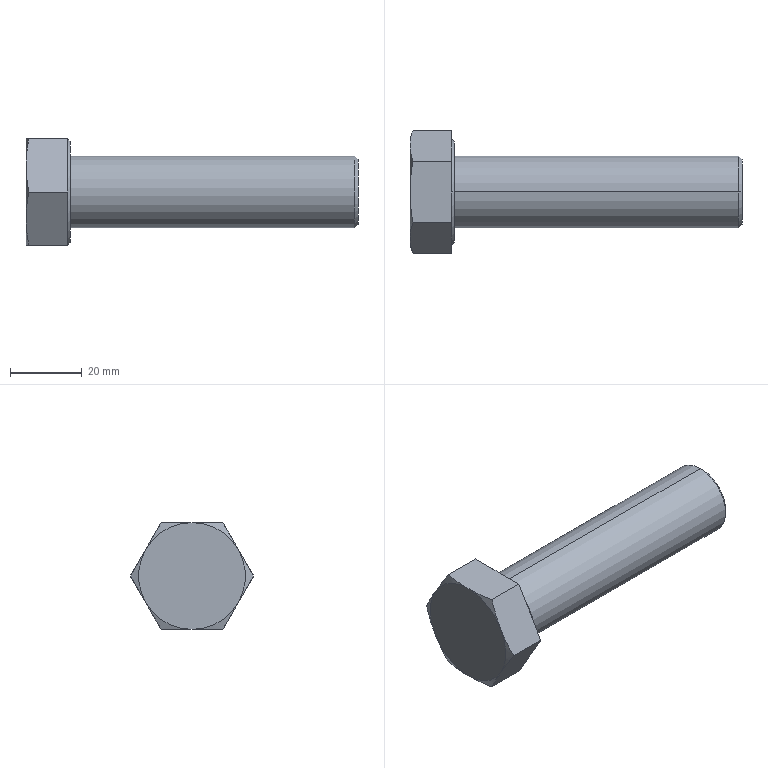Part | SolidWorks | features RevCut 3, Boss 1, Chamfer 1, Extrusion 1, Fillet 1, LPattern 1 | 1 solid | 27 faces | box 92.28 x 34.26 x 29.67 mm | volume 34365 mm3 | plane 15 | cone 10 | cylinder 2 | commonest cylinder face diameters 20 x2
STEP:
#1=CARTESIAN_POINT('',(92.28,0.,-9.));
#2=VERTEX_POINT('',#1);
#3=CARTESIAN_POINT('',(92.28,0.,9.));
#4=VERTEX_POINT('',#3);
#5=CARTESIAN_POINT('',(92.28,0.,0.));
#6=DIRECTION('',(1.,0.,0.));
#7=DIRECTION('',(0.,0.,-1.));
#8=AXIS2_PLACEMENT_3D('',#5,#6,#7);
#9=CIRCLE('',#8,9.);
#10=EDGE_CURVE('',#2,#4,#9,.T.);
#11=ORIENTED_EDGE('',*,*,#10,.F.);
#12=CARTESIAN_POINT('',(91.28,0.,-10.));
#13=VERTEX_POINT('',#12);
#14=CARTESIAN_POINT('',(92.28,0.,-9.));
#15=DIRECTION('',(-0.7071,0.,-0.7071));
#16=VECTOR('',#15,1000.);
#17=LINE('',#14,#16);
#18=EDGE_CURVE('',#2,#13,#17,.T.);
#19=ORIENTED_EDGE('',*,*,#18,.T.);
#20=CARTESIAN_POINT('',(91.28,0.,10.));
#21=VERTEX_POINT('',#20);
#22=CARTESIAN_POINT('',(91.28,0.,0.));
#23=DIRECTION('',(-1.,0.,0.));
#24=DIRECTION('',(0.,0.,-1.));
#25=AXIS2_PLACEMENT_3D('',#22,#23,#24);
#26=CIRCLE('',#25,10.);
#27=EDGE_CURVE('',#21,#13,#26,.T.);
#28=ORIENTED_EDGE('',*,*,#27,.F.);
#29=CARTESIAN_POINT('',(92.28,0.,9.));
#30=DIRECTION('',(-0.7071,0.,0.7071));
#31=VECTOR('',#30,1000.);
#32=LINE('',#29,#31);
#33=EDGE_CURVE('',#4,#21,#32,.T.);
#34=ORIENTED_EDGE('',*,*,#33,.F.);
#35=EDGE_LOOP('',(#11,#19,#28,#34));
#36=FACE_OUTER_BOUND('',#35,.T.);
#37=CARTESIAN_POINT('',(92.28,0.,0.));
#38=DIRECTION('',(-1.,0.,0.));
#39=DIRECTION('',(0.,0.,1.));
#40=AXIS2_PLACEMENT_3D('',#37,#38,#39);
#41=CONICAL_SURFACE('',#40,9.,0.7854);
#42=ADVANCED_FACE('',(#36),#41,.T.);
#43=ORIENTED_EDGE('',*,*,#27,.T.);
#44=CARTESIAN_POINT('',(12.28,0.,-10.));
#45=VERTEX_POINT('',#44);
#46=CARTESIAN_POINT('',(92.28,0.,-10.));
#47=DIRECTION('',(-1.,0.,0.));
#48=VECTOR('',#47,1000.);
#49=LINE('',#46,#48);
#50=EDGE_CURVE('',#13,#45,#49,.T.);
#51=ORIENTED_EDGE('',*,*,#50,.T.);
#52=CARTESIAN_POINT('',(12.28,0.,10.));
#53=VERTEX_POINT('',#52);
#54=CARTESIAN_POINT('',(12.28,0.,0.));
#55=DIRECTION('',(1.,0.,0.));
#56=DIRECTION('',(0.,0.,-1.));
#57=AXIS2_PLACEMENT_3D('',#54,#55,#56);
#58=CIRCLE('',#57,10.);
#59=EDGE_CURVE('',#45,#53,#58,.T.);
#60=ORIENTED_EDGE('',*,*,#59,.T.);
#61=CARTESIAN_POINT('',(92.28,0.,10.));
#62=DIRECTION('',(-1.,0.,0.));
#63=VECTOR('',#62,1000.);
#64=LINE('',#61,#63);
#65=EDGE_CURVE('',#21,#53,#64,.T.);
#66=ORIENTED_EDGE('',*,*,#65,.F.);
#67=EDGE_LOOP('',(#43,#51,#60,#66));
#68=FACE_OUTER_BOUND('',#67,.T.);
#69=CARTESIAN_POINT('',(92.28,0.,0.));
#70=DIRECTION('',(-1.,0.,0.));
#71=DIRECTION('',(0.,0.,1.));
#72=AXIS2_PLACEMENT_3D('',#69,#70,#71);
#73=CYLINDRICAL_SURFACE('',#72,10.);
#74=ADVANCED_FACE('',(#68),#73,.T.);
#75=CARTESIAN_POINT('',(12.28,0.,14.095));
#76=VERTEX_POINT('',#75);
#77=CARTESIAN_POINT('',(12.28,0.,-14.095));
#78=VERTEX_POINT('',#77);
#79=CARTESIAN_POINT('',(12.28,0.,0.));
#80=DIRECTION('',(-1.,0.,0.));
#81=DIRECTION('',(0.,0.,1.));
#82=AXIS2_PLACEMENT_3D('',#79,#80,#81);
#83=CIRCLE('',#82,14.095);
#84=EDGE_CURVE('',#76,#78,#83,.T.);
#85=ORIENTED_EDGE('',*,*,#84,.T.);
#86=CARTESIAN_POINT('',(11.54,0.,-14.835));
#87=VERTEX_POINT('',#86);
#88=CARTESIAN_POINT('',(11.48,0.,-14.895));
#89=DIRECTION('',(-0.7071,0.,-0.7071));
#90=VECTOR('',#89,1000.);
#91=LINE('',#88,#90);
#92=EDGE_CURVE('',#78,#87,#91,.T.);
#93=ORIENTED_EDGE('',*,*,#92,.T.);
#94=CARTESIAN_POINT('',(11.48,1.336,-14.835));
#95=VERTEX_POINT('',#94);
#96=CARTESIAN_POINT('',(11.54,0.,-14.835));
#97=CARTESIAN_POINT('',(11.54,0.4454,-14.835));
#98=CARTESIAN_POINT('',(11.52,0.8906,-14.835));
#99=CARTESIAN_POINT('',(11.48,1.336,-14.835));
#100=B_SPLINE_CURVE_WITH_KNOTS('',3,(#96,#97,#98,#99),.UNSPECIFIED.,.F.,.F.,(4,4),(0.008338,0.009669),.UNSPECIFIED.);
#101=EDGE_CURVE('',#87,#95,#100,.T.);
#102=ORIENTED_EDGE('',*,*,#101,.T.);
#103=CARTESIAN_POINT('',(11.48,12.18,-8.574));
#104=VERTEX_POINT('',#103);
#105=CARTESIAN_POINT('',(11.48,0.,0.));
#106=DIRECTION('',(-1.,0.,0.));
#107=DIRECTION('',(0.,0.,1.));
#108=AXIS2_PLACEMENT_3D('',#105,#106,#107);
#109=CIRCLE('',#108,14.895);
#110=EDGE_CURVE('',#104,#95,#109,.T.);
#111=ORIENTED_EDGE('',*,*,#110,.F.);
#112=CARTESIAN_POINT('',(11.48,13.515,-6.261));
#113=VERTEX_POINT('',#112);
#114=CARTESIAN_POINT('',(11.48,12.18,-8.574));
#115=CARTESIAN_POINT('',(11.56,12.625,-7.803));
#116=CARTESIAN_POINT('',(11.56,13.07,-7.032));
#117=CARTESIAN_POINT('',(11.48,13.515,-6.261));
#118=B_SPLINE_CURVE_WITH_KNOTS('',3,(#114,#115,#116,#117),.UNSPECIFIED.,.F.,.F.,(4,4),(0.000002229,0.002673),.UNSPECIFIED.);
#119=EDGE_CURVE('',#104,#113,#118,.T.);
#120=ORIENTED_EDGE('',*,*,#119,.T.);
#121=CARTESIAN_POINT('',(11.48,13.515,6.261));
#122=VERTEX_POINT('',#121);
#123=CARTESIAN_POINT('',(11.48,0.,0.));
#124=DIRECTION('',(-1.,0.,0.));
#125=DIRECTION('',(0.,0.,1.));
#126=AXIS2_PLACEMENT_3D('',#123,#124,#125);
#127=CIRCLE('',#126,14.895);
#128=EDGE_CURVE('',#122,#113,#127,.T.);
#129=ORIENTED_EDGE('',*,*,#128,.F.);
#130=CARTESIAN_POINT('',(11.48,12.18,8.574));
#131=VERTEX_POINT('',#130);
#132=CARTESIAN_POINT('',(11.48,13.515,6.261));
#133=CARTESIAN_POINT('',(11.56,13.07,7.032));
#134=CARTESIAN_POINT('',(11.56,12.625,7.803));
#135=CARTESIAN_POINT('',(11.48,12.18,8.574));
#136=B_SPLINE_CURVE_WITH_KNOTS('',3,(#132,#133,#134,#135),.UNSPECIFIED.,.F.,.F.,(4,4),(0.000002229,0.002673),.UNSPECIFIED.);
#137=EDGE_CURVE('',#122,#131,#136,.T.);
#138=ORIENTED_EDGE('',*,*,#137,.T.);
#139=CARTESIAN_POINT('',(11.48,1.336,14.835));
#140=VERTEX_POINT('',#139);
#141=CARTESIAN_POINT('',(11.48,0.,0.));
#142=DIRECTION('',(-1.,0.,0.));
#143=DIRECTION('',(0.,0.,1.));
#144=AXIS2_PLACEMENT_3D('',#141,#142,#143);
#145=CIRCLE('',#144,14.895);
#146=EDGE_CURVE('',#140,#131,#145,.T.);
#147=ORIENTED_EDGE('',*,*,#146,.F.);
#148=CARTESIAN_POINT('',(11.54,0.,14.835));
#149=VERTEX_POINT('',#148);
#150=CARTESIAN_POINT('',(11.48,1.336,14.835));
#151=CARTESIAN_POINT('',(11.52,0.8906,14.835));
#152=CARTESIAN_POINT('',(11.54,0.4454,14.835));
#153=CARTESIAN_POINT('',(11.54,0.,14.835));
#154=B_SPLINE_CURVE_WITH_KNOTS('',3,(#150,#151,#152,#153),.UNSPECIFIED.,.F.,.F.,(4,4),(0.007682,0.009012),.UNSPECIFIED.);
#155=EDGE_CURVE('',#140,#149,#154,.T.);
#156=ORIENTED_EDGE('',*,*,#155,.T.);
#157=CARTESIAN_POINT('',(11.48,0.,14.895));
#158=DIRECTION('',(-0.7071,0.,0.7071));
#159=VECTOR('',#158,1000.);
#160=LINE('',#157,#159);
#161=EDGE_CURVE('',#76,#149,#160,.T.);
#162=ORIENTED_EDGE('',*,*,#161,.F.);
#163=EDGE_LOOP('',(#85,#93,#102,#111,#120,#129,#138,#147,#156,#162));
#164=FACE_OUTER_BOUND('',#163,.T.);
#165=CARTESIAN_POINT('',(11.48,0.,0.));
#166=DIRECTION('',(-1.,0.,0.));
#167=DIRECTION('',(0.,0.,1.));
#168=AXIS2_PLACEMENT_3D('',#165,#166,#167);
#169=CONICAL_SURFACE('',#168,14.895,0.7854);
#170=ADVANCED_FACE('',(#164),#169,.T.);
#171=ORIENTED_EDGE('',*,*,#84,.F.);
#172=CARTESIAN_POINT('',(12.28,0.,0.));
#173=DIRECTION('',(-1.,0.,0.));
#174=DIRECTION('',(0.,0.,1.));
#175=AXIS2_PLACEMENT_3D('',#172,#173,#174);
#176=CIRCLE('',#175,14.095);
#177=EDGE_CURVE('',#78,#76,#176,.T.);
#178=ORIENTED_EDGE('',*,*,#177,.F.);
#179=EDGE_LOOP('',(#171,#178));
#180=FACE_OUTER_BOUND('',#179,.T.);
#181=CARTESIAN_POINT('',(12.28,0.,0.));
#182=DIRECTION('',(1.,0.,0.));
#183=DIRECTION('',(0.,0.,-1.));
#184=AXIS2_PLACEMENT_3D('',#181,#182,#183);
#185=CIRCLE('',#184,10.);
#186=EDGE_CURVE('',#53,#45,#185,.T.);
#187=ORIENTED_EDGE('',*,*,#186,.F.);
#188=ORIENTED_EDGE('',*,*,#59,.F.);
#189=EDGE_LOOP('',(#187,#188));
#190=FACE_BOUND('',#189,.T.);
#191=CARTESIAN_POINT('',(12.28,-25.695,-14.835));
#192=DIRECTION('',(1.,0.,0.));
#193=DIRECTION('',(0.,0.,-1.));
#194=AXIS2_PLACEMENT_3D('',#191,#192,#193);
#195=PLANE('',#194);
#196=ADVANCED_FACE('',(#180,#190),#195,.T.);
#197=CARTESIAN_POINT('',(0.8353,-17.13,0.));
#198=VERTEX_POINT('',#197);
#199=CARTESIAN_POINT('',(0.,-12.847,7.418));
#200=VERTEX_POINT('',#199);
#201=CARTESIAN_POINT('',(0.8353,-17.13,0.));
#202=CARTESIAN_POINT('',(0.5755,-16.416,1.236));
#203=CARTESIAN_POINT('',(0.3646,-15.702,2.473));
#204=CARTESIAN_POINT('',(0.07638,-14.275,4.945));
#205=CARTESIAN_POINT('',(0.,-13.561,6.181));
#206=CARTESIAN_POINT('',(0.,-12.847,7.418));
#207=B_SPLINE_CURVE_WITH_KNOTS('',3,(#201,#202,#203,#204,#205,#206),.UNSPECIFIED.,.F.,.F.,(4,2,4),(0.000000231,0.004283,0.008565),.UNSPECIFIED.);
#208=EDGE_CURVE('',#198,#200,#207,.T.);
#209=ORIENTED_EDGE('',*,*,#208,.F.);
#210=CARTESIAN_POINT('',(11.48,-17.13,0.));
#211=VERTEX_POINT('',#210);
#212=CARTESIAN_POINT('',(12.28,-17.13,0.));
#213=DIRECTION('',(-1.,0.,0.));
#214=VECTOR('',#213,1000.);
#215=LINE('',#212,#214);
#216=EDGE_CURVE('',#211,#198,#215,.T.);
#217=ORIENTED_EDGE('',*,*,#216,.F.);
#218=CARTESIAN_POINT('',(11.48,-13.515,6.261));
#219=VERTEX_POINT('',#218);
#220=CARTESIAN_POINT('',(11.48,-8.565,14.835));
#221=DIRECTION('',(0.,-0.5,-0.866));
#222=VECTOR('',#221,1000.);
#223=LINE('',#220,#222);
#224=EDGE_CURVE('',#219,#211,#223,.T.);
#225=ORIENTED_EDGE('',*,*,#224,.F.);
#226=CARTESIAN_POINT('',(11.48,-12.18,8.574));
#227=VERTEX_POINT('',#226);
#228=CARTESIAN_POINT('',(11.48,-12.18,8.574));
#229=CARTESIAN_POINT('',(11.56,-12.625,7.803));
#230=CARTESIAN_POINT('',(11.56,-13.07,7.032));
#231=CARTESIAN_POINT('',(11.48,-13.515,6.261));
#232=B_SPLINE_CURVE_WITH_KNOTS('',3,(#228,#229,#230,#231),.UNSPECIFIED.,.F.,.F.,(4,4),(0.000002229,0.002673),.UNSPECIFIED.);
#233=EDGE_CURVE('',#227,#219,#232,.T.);
#234=ORIENTED_EDGE('',*,*,#233,.F.);
#235=CARTESIAN_POINT('',(11.48,-8.565,14.835));
#236=VERTEX_POINT('',#235);
#237=CARTESIAN_POINT('',(11.48,-8.565,14.835));
#238=DIRECTION('',(0.,-0.5,-0.866));
#239=VECTOR('',#238,1000.);
#240=LINE('',#237,#239);
#241=EDGE_CURVE('',#236,#227,#240,.T.);
#242=ORIENTED_EDGE('',*,*,#241,.F.);
#243=CARTESIAN_POINT('',(0.8353,-8.565,14.835));
#244=VERTEX_POINT('',#243);
#245=CARTESIAN_POINT('',(12.28,-8.565,14.835));
#246=DIRECTION('',(-1.,0.,0.));
#247=VECTOR('',#246,1000.);
#248=LINE('',#245,#247);
#249=EDGE_CURVE('',#236,#244,#248,.T.);
#250=ORIENTED_EDGE('',*,*,#249,.T.);
#251=CARTESIAN_POINT('',(0.,-12.847,7.418));
#252=CARTESIAN_POINT('',(0.,-12.134,8.654));
#253=CARTESIAN_POINT('',(0.07638,-11.42,9.89));
#254=CARTESIAN_POINT('',(0.3646,-9.992,12.363));
#255=CARTESIAN_POINT('',(0.5755,-9.279,13.599));
#256=CARTESIAN_POINT('',(0.8353,-8.565,14.835));
#257=B_SPLINE_CURVE_WITH_KNOTS('',3,(#251,#252,#253,#254,#255,#256),.UNSPECIFIED.,.F.,.F.,(4,2,4),(0.008565,0.01285,0.01713),.UNSPECIFIED.);
#258=EDGE_CURVE('',#200,#244,#257,.T.);
#259=ORIENTED_EDGE('',*,*,#258,.F.);
#260=EDGE_LOOP('',(#209,#217,#225,#234,#242,#250,#259));
#261=FACE_OUTER_BOUND('',#260,.T.);
#262=CARTESIAN_POINT('',(12.28,-8.565,14.835));
#263=DIRECTION('',(0.,0.866,-0.5));
#264=DIRECTION('',(0.,0.5,0.866));
#265=AXIS2_PLACEMENT_3D('',#262,#263,#264);
#266=PLANE('',#265);
#267=ADVANCED_FACE('',(#261),#266,.F.);
#268=CARTESIAN_POINT('',(0.8353,-8.565,-14.835));
#269=VERTEX_POINT('',#268);
#270=CARTESIAN_POINT('',(0.,-12.847,-7.417));
#271=VERTEX_POINT('',#270);
#272=CARTESIAN_POINT('',(0.8353,-8.565,-14.835));
#273=CARTESIAN_POINT('',(0.5755,-9.279,-13.599));
#274=CARTESIAN_POINT('',(0.3646,-9.992,-12.363));
#275=CARTESIAN_POINT('',(0.07638,-11.42,-9.89));
#276=CARTESIAN_POINT('',(0.,-12.134,-8.654));
#277=CARTESIAN_POINT('',(0.,-12.847,-7.417));
#278=B_SPLINE_CURVE_WITH_KNOTS('',3,(#272,#273,#274,#275,#276,#277),.UNSPECIFIED.,.F.,.F.,(4,2,4),(0.000000231,0.004283,0.008565),.UNSPECIFIED.);
#279=EDGE_CURVE('',#269,#271,#278,.T.);
#280=ORIENTED_EDGE('',*,*,#279,.F.);
#281=CARTESIAN_POINT('',(11.48,-8.565,-14.835));
#282=VERTEX_POINT('',#281);
#283=CARTESIAN_POINT('',(12.28,-8.565,-14.835));
#284=DIRECTION('',(-1.,0.,0.));
#285=VECTOR('',#284,1000.);
#286=LINE('',#283,#285);
#287=EDGE_CURVE('',#282,#269,#286,.T.);
#288=ORIENTED_EDGE('',*,*,#287,.F.);
#289=CARTESIAN_POINT('',(11.48,-12.18,-8.574));
#290=VERTEX_POINT('',#289);
#291=CARTESIAN_POINT('',(11.48,-17.13,0.));
#292=DIRECTION('',(0.,0.5,-0.866));
#293=VECTOR('',#292,1000.);
#294=LINE('',#291,#293);
#295=EDGE_CURVE('',#290,#282,#294,.T.);
#296=ORIENTED_EDGE('',*,*,#295,.F.);
#297=CARTESIAN_POINT('',(11.48,-13.515,-6.261));
#298=VERTEX_POINT('',#297);
#299=CARTESIAN_POINT('',(11.48,-13.515,-6.261));
#300=CARTESIAN_POINT('',(11.56,-13.07,-7.032));
#301=CARTESIAN_POINT('',(11.56,-12.625,-7.803));
#302=CARTESIAN_POINT('',(11.48,-12.18,-8.574));
#303=B_SPLINE_CURVE_WITH_KNOTS('',3,(#299,#300,#301,#302),.UNSPECIFIED.,.F.,.F.,(4,4),(0.000002229,0.002673),.UNSPECIFIED.);
#304=EDGE_CURVE('',#298,#290,#303,.T.);
#305=ORIENTED_EDGE('',*,*,#304,.F.);
#306=CARTESIAN_POINT('',(11.48,-17.13,0.));
#307=DIRECTION('',(0.,0.5,-0.866));
#308=VECTOR('',#307,1000.);
#309=LINE('',#306,#308);
#310=EDGE_CURVE('',#211,#298,#309,.T.);
#311=ORIENTED_EDGE('',*,*,#310,.F.);
#312=ORIENTED_EDGE('',*,*,#216,.T.);
#313=CARTESIAN_POINT('',(0.,-12.847,-7.417));
#314=CARTESIAN_POINT('',(0.,-13.561,-6.181));
#315=CARTESIAN_POINT('',(0.07638,-14.275,-4.945));
#316=CARTESIAN_POINT('',(0.3646,-15.702,-2.473));
#317=CARTESIAN_POINT('',(0.5755,-16.416,-1.236));
#318=CARTESIAN_POINT('',(0.8353,-17.13,0.));
#319=B_SPLINE_CURVE_WITH_KNOTS('',3,(#313,#314,#315,#316,#317,#318),.UNSPECIFIED.,.F.,.F.,(4,2,4),(0.008565,0.01285,0.01713),.UNSPECIFIED.);
#320=EDGE_CURVE('',#271,#198,#319,.T.);
#321=ORIENTED_EDGE('',*,*,#320,.F.);
#322=EDGE_LOOP('',(#280,#288,#296,#305,#311,#312,#321));
#323=FACE_OUTER_BOUND('',#322,.T.);
#324=CARTESIAN_POINT('',(12.28,-17.13,0.));
#325=DIRECTION('',(0.,0.866,0.5));
#326=DIRECTION('',(0.,-0.5,0.866));
#327=AXIS2_PLACEMENT_3D('',#324,#325,#326);
#328=PLANE('',#327);
#329=ADVANCED_FACE('',(#323),#328,.F.);
#330=CARTESIAN_POINT('',(0.8353,8.565,-14.835));
#331=VERTEX_POINT('',#330);
#332=CARTESIAN_POINT('',(0.,0.,-14.835));
#333=VERTEX_POINT('',#332);
#334=CARTESIAN_POINT('',(0.8353,8.565,-14.835));
#335=CARTESIAN_POINT('',(0.5762,7.141,-14.835));
#336=CARTESIAN_POINT('',(0.3651,5.714,-14.835));
#337=CARTESIAN_POINT('',(0.07668,2.859,-14.835));
#338=CARTESIAN_POINT('',(0.,1.43,-14.835));
#339=CARTESIAN_POINT('',(0.,0.,-14.835));
#340=B_SPLINE_CURVE_WITH_KNOTS('',3,(#334,#335,#336,#337,#338,#339),.UNSPECIFIED.,.F.,.F.,(4,2,4),(0.03088,0.0352,0.03952),.UNSPECIFIED.);
#341=EDGE_CURVE('',#331,#333,#340,.T.);
#342=ORIENTED_EDGE('',*,*,#341,.F.);
#343=CARTESIAN_POINT('',(11.48,8.565,-14.835));
#344=VERTEX_POINT('',#343);
#345=CARTESIAN_POINT('',(12.28,8.565,-14.835));
#346=DIRECTION('',(-1.,0.,0.));
#347=VECTOR('',#346,1000.);
#348=LINE('',#345,#347);
#349=EDGE_CURVE('',#344,#331,#348,.T.);
#350=ORIENTED_EDGE('',*,*,#349,.F.);
#351=CARTESIAN_POINT('',(11.48,-8.565,-14.835));
#352=DIRECTION('',(0.,1.,0.));
#353=VECTOR('',#352,1000.);
#354=LINE('',#351,#353);
#355=EDGE_CURVE('',#95,#344,#354,.T.);
#356=ORIENTED_EDGE('',*,*,#355,.F.);
#357=ORIENTED_EDGE('',*,*,#101,.F.);
#358=CARTESIAN_POINT('',(11.48,-1.336,-14.835));
#359=VERTEX_POINT('',#358);
#360=CARTESIAN_POINT('',(11.48,-1.336,-14.835));
#361=CARTESIAN_POINT('',(11.52,-0.8902,-14.835));
#362=CARTESIAN_POINT('',(11.54,-0.445,-14.835));
#363=CARTESIAN_POINT('',(11.54,0.,-14.835));
#364=B_SPLINE_CURVE_WITH_KNOTS('',3,(#360,#361,#362,#363),.UNSPECIFIED.,.F.,.F.,(4,4),(0.007008,0.008338),.UNSPECIFIED.);
#365=EDGE_CURVE('',#359,#87,#364,.T.);
#366=ORIENTED_EDGE('',*,*,#365,.F.);
#367=CARTESIAN_POINT('',(11.48,-8.565,-14.835));
#368=DIRECTION('',(0.,1.,0.));
#369=VECTOR('',#368,1000.);
#370=LINE('',#367,#369);
#371=EDGE_CURVE('',#282,#359,#370,.T.);
#372=ORIENTED_EDGE('',*,*,#371,.F.);
#373=ORIENTED_EDGE('',*,*,#287,.T.);
#374=CARTESIAN_POINT('',(0.,0.,-14.835));
#375=CARTESIAN_POINT('',(0.,-1.426,-14.835));
#376=CARTESIAN_POINT('',(0.07627,-2.854,-14.835));
#377=CARTESIAN_POINT('',(0.3649,-5.713,-14.835));
#378=CARTESIAN_POINT('',(0.5772,-7.147,-14.835));
#379=CARTESIAN_POINT('',(0.8353,-8.565,-14.835));
#380=B_SPLINE_CURVE_WITH_KNOTS('',3,(#374,#375,#376,#377,#378,#379),.UNSPECIFIED.,.F.,.F.,(4,2,4),(0.03952,0.04383,0.04813),.UNSPECIFIED.);
#381=EDGE_CURVE('',#333,#269,#380,.T.);
#382=ORIENTED_EDGE('',*,*,#381,.F.);
#383=EDGE_LOOP('',(#342,#350,#356,#357,#366,#372,#373,#382));
#384=FACE_OUTER_BOUND('',#383,.T.);
#385=CARTESIAN_POINT('',(12.28,-8.565,-14.835));
#386=DIRECTION('',(0.,0.,1.));
#387=DIRECTION('',(1.,0.,0.));
#388=AXIS2_PLACEMENT_3D('',#385,#386,#387);
#389=PLANE('',#388);
#390=ADVANCED_FACE('',(#384),#389,.F.);
#391=CARTESIAN_POINT('',(0.8353,17.13,0.));
#392=VERTEX_POINT('',#391);
#393=CARTESIAN_POINT('',(0.,12.847,-7.417));
#394=VERTEX_POINT('',#393);
#395=CARTESIAN_POINT('',(0.8353,17.13,0.));
#396=CARTESIAN_POINT('',(0.5755,16.416,-1.236));
#397=CARTESIAN_POINT('',(0.3646,15.702,-2.473));
#398=CARTESIAN_POINT('',(0.07638,14.275,-4.945));
#399=CARTESIAN_POINT('',(0.,13.561,-6.181));
#400=CARTESIAN_POINT('',(0.,12.847,-7.417));
#401=B_SPLINE_CURVE_WITH_KNOTS('',3,(#395,#396,#397,#398,#399,#400),.UNSPECIFIED.,.F.,.F.,(4,2,4),(0.000000231,0.004283,0.008565),.UNSPECIFIED.);
#402=EDGE_CURVE('',#392,#394,#401,.T.);
#403=ORIENTED_EDGE('',*,*,#402,.F.);
#404=CARTESIAN_POINT('',(11.48,17.13,0.));
#405=VERTEX_POINT('',#404);
#406=CARTESIAN_POINT('',(12.28,17.13,0.));
#407=DIRECTION('',(-1.,0.,0.));
#408=VECTOR('',#407,1000.);
#409=LINE('',#406,#408);
#410=EDGE_CURVE('',#405,#392,#409,.T.);
#411=ORIENTED_EDGE('',*,*,#410,.F.);
#412=CARTESIAN_POINT('',(11.48,8.565,-14.835));
#413=DIRECTION('',(0.,0.5,0.866));
#414=VECTOR('',#413,1000.);
#415=LINE('',#412,#414);
#416=EDGE_CURVE('',#113,#405,#415,.T.);
#417=ORIENTED_EDGE('',*,*,#416,.F.);
#418=ORIENTED_EDGE('',*,*,#119,.F.);
#419=CARTESIAN_POINT('',(11.48,8.565,-14.835));
#420=DIRECTION('',(0.,0.5,0.866));
#421=VECTOR('',#420,1000.);
#422=LINE('',#419,#421);
#423=EDGE_CURVE('',#344,#104,#422,.T.);
#424=ORIENTED_EDGE('',*,*,#423,.F.);
#425=ORIENTED_EDGE('',*,*,#349,.T.);
#426=CARTESIAN_POINT('',(0.,12.847,-7.417));
#427=CARTESIAN_POINT('',(0.,12.134,-8.654));
#428=CARTESIAN_POINT('',(0.07638,11.42,-9.89));
#429=CARTESIAN_POINT('',(0.3646,9.992,-12.362));
#430=CARTESIAN_POINT('',(0.5755,9.279,-13.599));
#431=CARTESIAN_POINT('',(0.8353,8.565,-14.835));
#432=B_SPLINE_CURVE_WITH_KNOTS('',3,(#426,#427,#428,#429,#430,#431),.UNSPECIFIED.,.F.,.F.,(4,2,4),(0.008565,0.01285,0.01713),.UNSPECIFIED.);
#433=EDGE_CURVE('',#394,#331,#432,.T.);
#434=ORIENTED_EDGE('',*,*,#433,.F.);
#435=EDGE_LOOP('',(#403,#411,#417,#418,#424,#425,#434));
#436=FACE_OUTER_BOUND('',#435,.T.);
#437=CARTESIAN_POINT('',(12.28,8.565,-14.835));
#438=DIRECTION('',(0.,-0.866,0.5));
#439=DIRECTION('',(0.,-0.5,-0.866));
#440=AXIS2_PLACEMENT_3D('',#437,#438,#439);
#441=PLANE('',#440);
#442=ADVANCED_FACE('',(#436),#441,.F.);
#443=CARTESIAN_POINT('',(0.8353,8.565,14.835));
#444=VERTEX_POINT('',#443);
#445=CARTESIAN_POINT('',(0.,12.847,7.417));
#446=VERTEX_POINT('',#445);
#447=CARTESIAN_POINT('',(0.8353,8.565,14.835));
#448=CARTESIAN_POINT('',(0.5755,9.279,13.599));
#449=CARTESIAN_POINT('',(0.3646,9.992,12.363));
#450=CARTESIAN_POINT('',(0.07638,11.42,9.89));
#451=CARTESIAN_POINT('',(0.,12.134,8.654));
#452=CARTESIAN_POINT('',(0.,12.847,7.417));
#453=B_SPLINE_CURVE_WITH_KNOTS('',3,(#447,#448,#449,#450,#451,#452),.UNSPECIFIED.,.F.,.F.,(4,2,4),(0.000000231,0.004283,0.008565),.UNSPECIFIED.);
#454=EDGE_CURVE('',#444,#446,#453,.T.);
#455=ORIENTED_EDGE('',*,*,#454,.F.);
#456=CARTESIAN_POINT('',(11.48,8.565,14.835));
#457=VERTEX_POINT('',#456);
#458=CARTESIAN_POINT('',(12.28,8.565,14.835));
#459=DIRECTION('',(-1.,0.,0.));
#460=VECTOR('',#459,1000.);
#461=LINE('',#458,#460);
#462=EDGE_CURVE('',#457,#444,#461,.T.);
#463=ORIENTED_EDGE('',*,*,#462,.F.);
#464=CARTESIAN_POINT('',(11.48,17.13,0.));
#465=DIRECTION('',(0.,-0.5,0.866));
#466=VECTOR('',#465,1000.);
#467=LINE('',#464,#466);
#468=EDGE_CURVE('',#131,#457,#467,.T.);
#469=ORIENTED_EDGE('',*,*,#468,.F.);
#470=ORIENTED_EDGE('',*,*,#137,.F.);
#471=CARTESIAN_POINT('',(11.48,17.13,0.));
#472=DIRECTION('',(0.,-0.5,0.866));
#473=VECTOR('',#472,1000.);
#474=LINE('',#471,#473);
#475=EDGE_CURVE('',#405,#122,#474,.T.);
#476=ORIENTED_EDGE('',*,*,#475,.F.);
#477=ORIENTED_EDGE('',*,*,#410,.T.);
#478=CARTESIAN_POINT('',(0.,12.847,7.417));
#479=CARTESIAN_POINT('',(0.,13.561,6.181));
#480=CARTESIAN_POINT('',(0.07638,14.275,4.945));
#481=CARTESIAN_POINT('',(0.3646,15.702,2.472));
#482=CARTESIAN_POINT('',(0.5755,16.416,1.236));
#483=CARTESIAN_POINT('',(0.8353,17.13,0.));
#484=B_SPLINE_CURVE_WITH_KNOTS('',3,(#478,#479,#480,#481,#482,#483),.UNSPECIFIED.,.F.,.F.,(4,2,4),(0.008565,0.01285,0.01713),.UNSPECIFIED.);
#485=EDGE_CURVE('',#446,#392,#484,.T.);
#486=ORIENTED_EDGE('',*,*,#485,.F.);
#487=EDGE_LOOP('',(#455,#463,#469,#470,#476,#477,#486));
#488=FACE_OUTER_BOUND('',#487,.T.);
#489=CARTESIAN_POINT('',(12.28,17.13,0.));
#490=DIRECTION('',(0.,-0.866,-0.5));
#491=DIRECTION('',(0.,0.5,-0.866));
#492=AXIS2_PLACEMENT_3D('',#489,#490,#491);
#493=PLANE('',#492);
#494=ADVANCED_FACE('',(#488),#493,.F.);
#495=CARTESIAN_POINT('',(0.,0.,14.835));
#496=VERTEX_POINT('',#495);
#497=CARTESIAN_POINT('',(0.8353,-8.565,14.835));
#498=CARTESIAN_POINT('',(0.5772,-7.147,14.835));
#499=CARTESIAN_POINT('',(0.3649,-5.713,14.835));
#500=CARTESIAN_POINT('',(0.07627,-2.854,14.835));
#501=CARTESIAN_POINT('',(0.,-1.426,14.835));
#502=CARTESIAN_POINT('',(0.,0.,14.835));
#503=B_SPLINE_CURVE_WITH_KNOTS('',3,(#497,#498,#499,#500,#501,#502),.UNSPECIFIED.,.F.,.F.,(4,2,4),(0.01457,0.01889,0.0232),.UNSPECIFIED.);
#504=EDGE_CURVE('',#244,#496,#503,.T.);
#505=ORIENTED_EDGE('',*,*,#504,.F.);
#506=ORIENTED_EDGE('',*,*,#249,.F.);
#507=CARTESIAN_POINT('',(11.48,-1.336,14.835));
#508=VERTEX_POINT('',#507);
#509=CARTESIAN_POINT('',(11.48,8.565,14.835));
#510=DIRECTION('',(0.,-1.,0.));
#511=VECTOR('',#510,1000.);
#512=LINE('',#509,#511);
#513=EDGE_CURVE('',#508,#236,#512,.T.);
#514=ORIENTED_EDGE('',*,*,#513,.F.);
#515=CARTESIAN_POINT('',(11.54,0.,14.835));
#516=CARTESIAN_POINT('',(11.54,-0.445,14.835));
#517=CARTESIAN_POINT('',(11.52,-0.8902,14.835));
#518=CARTESIAN_POINT('',(11.48,-1.336,14.835));
#519=B_SPLINE_CURVE_WITH_KNOTS('',3,(#515,#516,#517,#518),.UNSPECIFIED.,.F.,.F.,(4,4),(0.009012,0.01034),.UNSPECIFIED.);
#520=EDGE_CURVE('',#149,#508,#519,.T.);
#521=ORIENTED_EDGE('',*,*,#520,.F.);
#522=ORIENTED_EDGE('',*,*,#155,.F.);
#523=CARTESIAN_POINT('',(11.48,8.565,14.835));
#524=DIRECTION('',(0.,-1.,0.));
#525=VECTOR('',#524,1000.);
#526=LINE('',#523,#525);
#527=EDGE_CURVE('',#457,#140,#526,.T.);
#528=ORIENTED_EDGE('',*,*,#527,.F.);
#529=ORIENTED_EDGE('',*,*,#462,.T.);
#530=CARTESIAN_POINT('',(0.,0.,14.835));
#531=CARTESIAN_POINT('',(0.,1.43,14.835));
#532=CARTESIAN_POINT('',(0.07668,2.859,14.835));
#533=CARTESIAN_POINT('',(0.3651,5.714,14.835));
#534=CARTESIAN_POINT('',(0.5762,7.141,14.835));
#535=CARTESIAN_POINT('',(0.8353,8.565,14.835));
#536=B_SPLINE_CURVE_WITH_KNOTS('',3,(#530,#531,#532,#533,#534,#535),.UNSPECIFIED.,.F.,.F.,(4,2,4),(0.0232,0.02753,0.03186),.UNSPECIFIED.);
#537=EDGE_CURVE('',#496,#444,#536,.T.);
#538=ORIENTED_EDGE('',*,*,#537,.F.);
#539=EDGE_LOOP('',(#505,#506,#514,#521,#522,#528,#529,#538));
#540=FACE_OUTER_BOUND('',#539,.T.);
#541=CARTESIAN_POINT('',(12.28,8.565,14.835));
#542=DIRECTION('',(0.,0.,-1.));
#543=DIRECTION('',(-1.,0.,0.));
#544=AXIS2_PLACEMENT_3D('',#541,#542,#543);
#545=PLANE('',#544);
#546=ADVANCED_FACE('',(#540),#545,.F.);
#547=ORIENTED_EDGE('',*,*,#224,.T.);
#548=ORIENTED_EDGE('',*,*,#310,.T.);
#549=CARTESIAN_POINT('',(11.48,0.,0.));
#550=DIRECTION('',(-1.,0.,0.));
#551=DIRECTION('',(0.,0.,1.));
#552=AXIS2_PLACEMENT_3D('',#549,#550,#551);
#553=CIRCLE('',#552,14.895);
#554=EDGE_CURVE('',#298,#219,#553,.T.);
#555=ORIENTED_EDGE('',*,*,#554,.T.);
#556=EDGE_LOOP('',(#547,#548,#555));
#557=FACE_OUTER_BOUND('',#556,.T.);
#558=CARTESIAN_POINT('',(11.48,14.895,0.));
#559=DIRECTION('',(1.,0.,0.));
#560=DIRECTION('',(0.,0.,-1.));
#561=AXIS2_PLACEMENT_3D('',#558,#559,#560);
#562=PLANE('',#561);
#563=ADVANCED_FACE('',(#557),#562,.T.);
#564=ORIENTED_EDGE('',*,*,#295,.T.);
#565=ORIENTED_EDGE('',*,*,#371,.T.);
#566=CARTESIAN_POINT('',(11.48,0.,0.));
#567=DIRECTION('',(-1.,0.,0.));
#568=DIRECTION('',(0.,0.,1.));
#569=AXIS2_PLACEMENT_3D('',#566,#567,#568);
#570=CIRCLE('',#569,14.895);
#571=EDGE_CURVE('',#359,#290,#570,.T.);
#572=ORIENTED_EDGE('',*,*,#571,.T.);
#573=EDGE_LOOP('',(#564,#565,#572));
#574=FACE_OUTER_BOUND('',#573,.T.);
#575=CARTESIAN_POINT('',(11.48,14.895,0.));
#576=DIRECTION('',(1.,0.,0.));
#577=DIRECTION('',(0.,0.,-1.));
#578=AXIS2_PLACEMENT_3D('',#575,#576,#577);
#579=PLANE('',#578);
#580=ADVANCED_FACE('',(#574),#579,.T.);
#581=ORIENTED_EDGE('',*,*,#355,.T.);
#582=ORIENTED_EDGE('',*,*,#423,.T.);
#583=ORIENTED_EDGE('',*,*,#110,.T.);
#584=EDGE_LOOP('',(#581,#582,#583));
#585=FACE_OUTER_BOUND('',#584,.T.);
#586=CARTESIAN_POINT('',(11.48,14.895,0.));
#587=DIRECTION('',(1.,0.,0.));
#588=DIRECTION('',(0.,0.,-1.));
#589=AXIS2_PLACEMENT_3D('',#586,#587,#588);
#590=PLANE('',#589);
#591=ADVANCED_FACE('',(#585),#590,.T.);
#592=ORIENTED_EDGE('',*,*,#416,.T.);
#593=ORIENTED_EDGE('',*,*,#475,.T.);
#594=ORIENTED_EDGE('',*,*,#128,.T.);
#595=EDGE_LOOP('',(#592,#593,#594));
#596=FACE_OUTER_BOUND('',#595,.T.);
#597=CARTESIAN_POINT('',(11.48,14.895,0.));
#598=DIRECTION('',(1.,0.,0.));
#599=DIRECTION('',(0.,0.,-1.));
#600=AXIS2_PLACEMENT_3D('',#597,#598,#599);
#601=PLANE('',#600);
#602=ADVANCED_FACE('',(#596),#601,.T.);
#603=ORIENTED_EDGE('',*,*,#468,.T.);
#604=ORIENTED_EDGE('',*,*,#527,.T.);
#605=ORIENTED_EDGE('',*,*,#146,.T.);
#606=EDGE_LOOP('',(#603,#604,#605));
#607=FACE_OUTER_BOUND('',#606,.T.);
#608=CARTESIAN_POINT('',(11.48,14.895,0.));
#609=DIRECTION('',(1.,0.,0.));
#610=DIRECTION('',(0.,0.,-1.));
#611=AXIS2_PLACEMENT_3D('',#608,#609,#610);
#612=PLANE('',#611);
#613=ADVANCED_FACE('',(#607),#612,.T.);
#614=ORIENTED_EDGE('',*,*,#241,.T.);
#615=CARTESIAN_POINT('',(11.48,0.,0.));
#616=DIRECTION('',(-1.,0.,0.));
#617=DIRECTION('',(0.,0.,1.));
#618=AXIS2_PLACEMENT_3D('',#615,#616,#617);
#619=CIRCLE('',#618,14.895);
#620=EDGE_CURVE('',#227,#508,#619,.T.);
#621=ORIENTED_EDGE('',*,*,#620,.T.);
#622=ORIENTED_EDGE('',*,*,#513,.T.);
#623=EDGE_LOOP('',(#614,#621,#622));
#624=FACE_OUTER_BOUND('',#623,.T.);
#625=CARTESIAN_POINT('',(11.48,14.895,0.));
#626=DIRECTION('',(1.,0.,0.));
#627=DIRECTION('',(0.,0.,-1.));
#628=AXIS2_PLACEMENT_3D('',#625,#626,#627);
#629=PLANE('',#628);
#630=ADVANCED_FACE('',(#624),#629,.T.);
#631=ORIENTED_EDGE('',*,*,#92,.F.);
#632=ORIENTED_EDGE('',*,*,#177,.T.);
#633=ORIENTED_EDGE('',*,*,#161,.T.);
#634=ORIENTED_EDGE('',*,*,#520,.T.);
#635=ORIENTED_EDGE('',*,*,#620,.F.);
#636=ORIENTED_EDGE('',*,*,#233,.T.);
#637=ORIENTED_EDGE('',*,*,#554,.F.);
#638=ORIENTED_EDGE('',*,*,#304,.T.);
#639=ORIENTED_EDGE('',*,*,#571,.F.);
#640=ORIENTED_EDGE('',*,*,#365,.T.);
#641=EDGE_LOOP('',(#631,#632,#633,#634,#635,#636,#637,#638,#639,#640));
#642=FACE_OUTER_BOUND('',#641,.T.);
#643=CARTESIAN_POINT('',(11.48,0.,0.));
#644=DIRECTION('',(-1.,0.,0.));
#645=DIRECTION('',(0.,0.,1.));
#646=AXIS2_PLACEMENT_3D('',#643,#644,#645);
#647=CONICAL_SURFACE('',#646,14.895,0.7854);
#648=ADVANCED_FACE('',(#642),#647,.T.);
#649=ORIENTED_EDGE('',*,*,#381,.T.);
#650=ORIENTED_EDGE('',*,*,#279,.T.);
#651=CARTESIAN_POINT('',(0.,0.,0.));
#652=DIRECTION('',(1.,0.,0.));
#653=DIRECTION('',(0.,0.,-1.));
#654=AXIS2_PLACEMENT_3D('',#651,#652,#653);
#655=CIRCLE('',#654,14.835);
#656=EDGE_CURVE('',#271,#333,#655,.T.);
#657=ORIENTED_EDGE('',*,*,#656,.T.);
#658=EDGE_LOOP('',(#649,#650,#657));
#659=FACE_OUTER_BOUND('',#658,.T.);
#660=CARTESIAN_POINT('',(0.,0.,0.));
#661=DIRECTION('',(1.,0.,0.));
#662=DIRECTION('',(0.,0.,-1.));
#663=AXIS2_PLACEMENT_3D('',#660,#661,#662);
#664=CONICAL_SURFACE('',#663,14.835,1.222);
#665=ADVANCED_FACE('',(#659),#664,.T.);
#666=ORIENTED_EDGE('',*,*,#320,.T.);
#667=ORIENTED_EDGE('',*,*,#208,.T.);
#668=CARTESIAN_POINT('',(0.,0.,0.));
#669=DIRECTION('',(1.,0.,0.));
#670=DIRECTION('',(0.,0.,-1.));
#671=AXIS2_PLACEMENT_3D('',#668,#669,#670);
#672=CIRCLE('',#671,14.835);
#673=EDGE_CURVE('',#200,#271,#672,.T.);
#674=ORIENTED_EDGE('',*,*,#673,.T.);
#675=EDGE_LOOP('',(#666,#667,#674));
#676=FACE_OUTER_BOUND('',#675,.T.);
#677=CARTESIAN_POINT('',(0.,0.,0.));
#678=DIRECTION('',(1.,0.,0.));
#679=DIRECTION('',(0.,0.,-1.));
#680=AXIS2_PLACEMENT_3D('',#677,#678,#679);
#681=CONICAL_SURFACE('',#680,14.835,1.222);
#682=ADVANCED_FACE('',(#676),#681,.T.);
#683=ORIENTED_EDGE('',*,*,#258,.T.);
#684=ORIENTED_EDGE('',*,*,#504,.T.);
#685=CARTESIAN_POINT('',(0.,0.,0.));
#686=DIRECTION('',(1.,0.,0.));
#687=DIRECTION('',(0.,0.,-1.));
#688=AXIS2_PLACEMENT_3D('',#685,#686,#687);
#689=CIRCLE('',#688,14.835);
#690=EDGE_CURVE('',#496,#200,#689,.T.);
#691=ORIENTED_EDGE('',*,*,#690,.T.);
#692=EDGE_LOOP('',(#683,#684,#691));
#693=FACE_OUTER_BOUND('',#692,.T.);
#694=CARTESIAN_POINT('',(0.,0.,0.));
#695=DIRECTION('',(1.,0.,0.));
#696=DIRECTION('',(0.,0.,-1.));
#697=AXIS2_PLACEMENT_3D('',#694,#695,#696);
#698=CONICAL_SURFACE('',#697,14.835,1.222);
#699=ADVANCED_FACE('',(#693),#698,.T.);
#700=ORIENTED_EDGE('',*,*,#454,.T.);
#701=CARTESIAN_POINT('',(0.,0.,0.));
#702=DIRECTION('',(-1.,0.,0.));
#703=DIRECTION('',(0.,0.,1.));
#704=AXIS2_PLACEMENT_3D('',#701,#702,#703);
#705=CIRCLE('',#704,14.835);
#706=EDGE_CURVE('',#496,#446,#705,.T.);
#707=ORIENTED_EDGE('',*,*,#706,.F.);
#708=ORIENTED_EDGE('',*,*,#537,.T.);
#709=EDGE_LOOP('',(#700,#707,#708));
#710=FACE_OUTER_BOUND('',#709,.T.);
#711=CARTESIAN_POINT('',(0.,0.,0.));
#712=DIRECTION('',(1.,0.,0.));
#713=DIRECTION('',(0.,0.,-1.));
#714=AXIS2_PLACEMENT_3D('',#711,#712,#713);
#715=CONICAL_SURFACE('',#714,14.835,1.222);
#716=ADVANCED_FACE('',(#710),#715,.T.);
#717=ORIENTED_EDGE('',*,*,#402,.T.);
#718=CARTESIAN_POINT('',(0.,0.,0.));
#719=DIRECTION('',(1.,0.,0.));
#720=DIRECTION('',(0.,0.,-1.));
#721=AXIS2_PLACEMENT_3D('',#718,#719,#720);
#722=CIRCLE('',#721,14.835);
#723=EDGE_CURVE('',#394,#446,#722,.T.);
#724=ORIENTED_EDGE('',*,*,#723,.T.);
#725=ORIENTED_EDGE('',*,*,#485,.T.);
#726=EDGE_LOOP('',(#717,#724,#725));
#727=FACE_OUTER_BOUND('',#726,.T.);
#728=CARTESIAN_POINT('',(0.,0.,0.));
#729=DIRECTION('',(1.,0.,0.));
#730=DIRECTION('',(0.,0.,-1.));
#731=AXIS2_PLACEMENT_3D('',#728,#729,#730);
#732=CONICAL_SURFACE('',#731,14.835,1.222);
#733=ADVANCED_FACE('',(#727),#732,.T.);
#734=ORIENTED_EDGE('',*,*,#341,.T.);
#735=CARTESIAN_POINT('',(0.,0.,0.));
#736=DIRECTION('',(1.,0.,0.));
#737=DIRECTION('',(0.,0.,-1.));
#738=AXIS2_PLACEMENT_3D('',#735,#736,#737);
#739=CIRCLE('',#738,14.835);
#740=EDGE_CURVE('',#333,#394,#739,.T.);
#741=ORIENTED_EDGE('',*,*,#740,.T.);
#742=ORIENTED_EDGE('',*,*,#433,.T.);
#743=EDGE_LOOP('',(#734,#741,#742));
#744=FACE_OUTER_BOUND('',#743,.T.);
#745=CARTESIAN_POINT('',(0.,0.,0.));
#746=DIRECTION('',(1.,0.,0.));
#747=DIRECTION('',(0.,0.,-1.));
#748=AXIS2_PLACEMENT_3D('',#745,#746,#747);
#749=CONICAL_SURFACE('',#748,14.835,1.222);
#750=ADVANCED_FACE('',(#744),#749,.T.);
#751=ORIENTED_EDGE('',*,*,#740,.F.);
#752=ORIENTED_EDGE('',*,*,#656,.F.);
#753=ORIENTED_EDGE('',*,*,#673,.F.);
#754=ORIENTED_EDGE('',*,*,#690,.F.);
#755=ORIENTED_EDGE('',*,*,#706,.T.);
#756=ORIENTED_EDGE('',*,*,#723,.F.);
#757=EDGE_LOOP('',(#751,#752,#753,#754,#755,#756));
#758=FACE_OUTER_BOUND('',#757,.T.);
#759=CARTESIAN_POINT('',(0.,-25.695,-14.835));
#760=DIRECTION('',(1.,0.,0.));
#761=DIRECTION('',(0.,0.,-1.));
#762=AXIS2_PLACEMENT_3D('',#759,#760,#761);
#763=PLANE('',#762);
#764=ADVANCED_FACE('',(#758),#763,.F.);
#765=ORIENTED_EDGE('',*,*,#50,.F.);
#766=CARTESIAN_POINT('',(91.28,0.,0.));
#767=DIRECTION('',(-1.,0.,0.));
#768=DIRECTION('',(0.,0.,-1.));
#769=AXIS2_PLACEMENT_3D('',#766,#767,#768);
#770=CIRCLE('',#769,10.);
#771=EDGE_CURVE('',#13,#21,#770,.T.);
#772=ORIENTED_EDGE('',*,*,#771,.T.);
#773=ORIENTED_EDGE('',*,*,#65,.T.);
#774=ORIENTED_EDGE('',*,*,#186,.T.);
#775=EDGE_LOOP('',(#765,#772,#773,#774));
#776=FACE_OUTER_BOUND('',#775,.T.);
#777=CARTESIAN_POINT('',(92.28,0.,0.));
#778=DIRECTION('',(-1.,0.,0.));
#779=DIRECTION('',(0.,0.,1.));
#780=AXIS2_PLACEMENT_3D('',#777,#778,#779);
#781=CYLINDRICAL_SURFACE('',#780,10.);
#782=ADVANCED_FACE('',(#776),#781,.T.);
#783=CARTESIAN_POINT('',(92.28,0.,0.));
#784=DIRECTION('',(1.,0.,0.));
#785=DIRECTION('',(0.,0.,-1.));
#786=AXIS2_PLACEMENT_3D('',#783,#784,#785);
#787=CIRCLE('',#786,9.);
#788=EDGE_CURVE('',#4,#2,#787,.T.);
#789=ORIENTED_EDGE('',*,*,#788,.T.);
#790=ORIENTED_EDGE('',*,*,#10,.T.);
#791=EDGE_LOOP('',(#789,#790));
#792=FACE_OUTER_BOUND('',#791,.T.);
#793=CARTESIAN_POINT('',(92.28,0.,0.));
#794=DIRECTION('',(1.,0.,0.));
#795=DIRECTION('',(0.,0.,-1.));
#796=AXIS2_PLACEMENT_3D('',#793,#794,#795);
#797=PLANE('',#796);
#798=ADVANCED_FACE('',(#792),#797,.T.);
#799=ORIENTED_EDGE('',*,*,#18,.F.);
#800=ORIENTED_EDGE('',*,*,#788,.F.);
#801=ORIENTED_EDGE('',*,*,#33,.T.);
#802=ORIENTED_EDGE('',*,*,#771,.F.);
#803=EDGE_LOOP('',(#799,#800,#801,#802));
#804=FACE_OUTER_BOUND('',#803,.T.);
#805=CARTESIAN_POINT('',(92.28,0.,0.));
#806=DIRECTION('',(-1.,0.,0.));
#807=DIRECTION('',(0.,0.,1.));
#808=AXIS2_PLACEMENT_3D('',#805,#806,#807);
#809=CONICAL_SURFACE('',#808,9.,0.7854);
#810=ADVANCED_FACE('',(#804),#809,.T.);
#811=CLOSED_SHELL('',(#42,#74,#170,#196,#267,#329,#390,#442,#494,#546,#563,#580,#591,#602,#613,#630,#648,#665,#682,#699,#716,#733,#750,#764,#782,#798,#810));
#812=MANIFOLD_SOLID_BREP('',#811);
#813=CARTESIAN_POINT('',(0.,0.,0.));
#814=DIRECTION('',(0.,0.,1.));
#815=DIRECTION('',(1.,0.,0.));
#816=AXIS2_PLACEMENT_3D('',#813,#814,#815);
#817=(LENGTH_UNIT()NAMED_UNIT(*)SI_UNIT(.MILLI.,.METRE.));
#818=UNCERTAINTY_MEASURE_WITH_UNIT(LENGTH_MEASURE(0.00001),#817,'','');
#819=(NAMED_UNIT(*)PLANE_ANGLE_UNIT()SI_UNIT($,.RADIAN.));
#820=(NAMED_UNIT(*)SI_UNIT($,.STERADIAN.)SOLID_ANGLE_UNIT());
#821=(GEOMETRIC_REPRESENTATION_CONTEXT(3)GLOBAL_UNCERTAINTY_ASSIGNED_CONTEXT((#818))GLOBAL_UNIT_ASSIGNED_CONTEXT((#817,#819,#820))REPRESENTATION_CONTEXT('',''));
#822=ADVANCED_BREP_SHAPE_REPRESENTATION('',(#812,#816),#821);